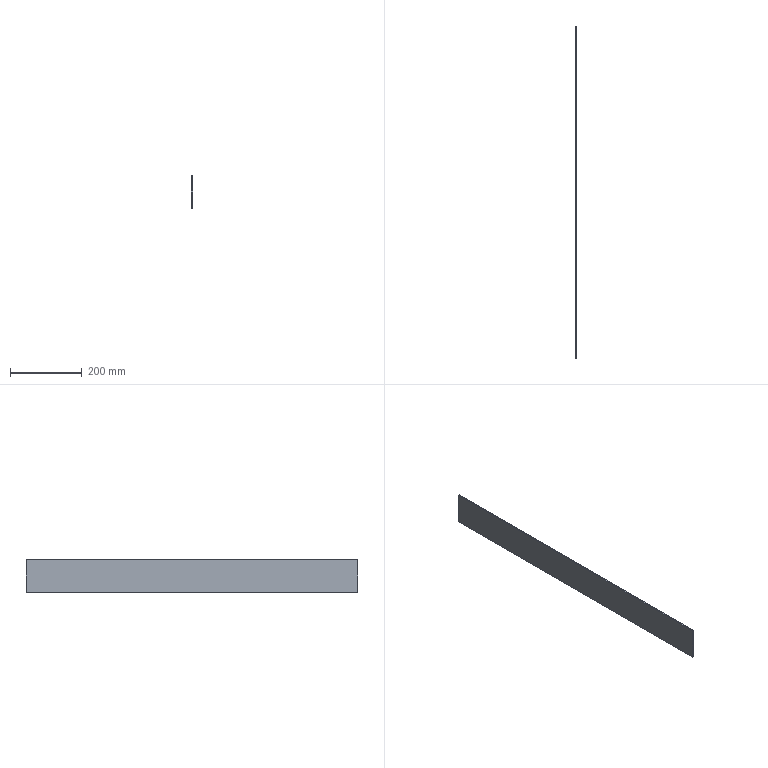Part | NX | features DATUM_CSYS 1, EXTRUDE 1, LINKED_CURVE 1 | 1 solid | 6 faces | box 3 x 926 x 90 mm | volume 250020 mm3 | plane 6
STEP:
#1=CARTESIAN_POINT('',(-455.,-463.,-88.163));
#2=VERTEX_POINT('',#1);
#3=CARTESIAN_POINT('',(-458.,-463.,-88.163));
#4=VERTEX_POINT('',#3);
#5=CARTESIAN_POINT('',(-455.,-463.,-88.163));
#6=DIRECTION('',(-1.,0.,0.));
#7=VECTOR('',#6,1000.);
#8=LINE('',#5,#7);
#9=EDGE_CURVE('',#2,#4,#8,.T.);
#10=ORIENTED_EDGE('',*,*,#9,.F.);
#11=CARTESIAN_POINT('',(-455.,-463.,1.837));
#12=VERTEX_POINT('',#11);
#13=CARTESIAN_POINT('',(-455.,-463.,-88.163));
#14=DIRECTION('',(0.,0.,1.));
#15=VECTOR('',#14,1000.);
#16=LINE('',#13,#15);
#17=EDGE_CURVE('',#2,#12,#16,.T.);
#18=ORIENTED_EDGE('',*,*,#17,.T.);
#19=CARTESIAN_POINT('',(-458.,-463.,1.837));
#20=VERTEX_POINT('',#19);
#21=CARTESIAN_POINT('',(-455.,-463.,1.837));
#22=DIRECTION('',(-1.,0.,0.));
#23=VECTOR('',#22,1000.);
#24=LINE('',#21,#23);
#25=EDGE_CURVE('',#12,#20,#24,.T.);
#26=ORIENTED_EDGE('',*,*,#25,.T.);
#27=CARTESIAN_POINT('',(-458.,-463.,-88.163));
#28=DIRECTION('',(0.,0.,1.));
#29=VECTOR('',#28,1000.);
#30=LINE('',#27,#29);
#31=EDGE_CURVE('',#4,#20,#30,.T.);
#32=ORIENTED_EDGE('',*,*,#31,.F.);
#33=EDGE_LOOP('',(#10,#18,#26,#32));
#34=FACE_BOUND('',#33,.T.);
#35=CARTESIAN_POINT('',(-455.,-463.,-88.163));
#36=DIRECTION('',(0.,-1.,0.));
#37=DIRECTION('',(0.,0.,1.));
#38=AXIS2_PLACEMENT_3D('',#35,#36,#37);
#39=PLANE('',#38);
#40=ADVANCED_FACE('',(#34),#39,.T.);
#41=ORIENTED_EDGE('',*,*,#25,.F.);
#42=CARTESIAN_POINT('',(-455.,463.,1.837));
#43=VERTEX_POINT('',#42);
#44=CARTESIAN_POINT('',(-455.,-463.,1.837));
#45=DIRECTION('',(0.,1.,0.));
#46=VECTOR('',#45,1000.);
#47=LINE('',#44,#46);
#48=EDGE_CURVE('',#12,#43,#47,.T.);
#49=ORIENTED_EDGE('',*,*,#48,.T.);
#50=CARTESIAN_POINT('',(-458.,463.,1.837));
#51=VERTEX_POINT('',#50);
#52=CARTESIAN_POINT('',(-455.,463.,1.837));
#53=DIRECTION('',(-1.,0.,0.));
#54=VECTOR('',#53,1000.);
#55=LINE('',#52,#54);
#56=EDGE_CURVE('',#43,#51,#55,.T.);
#57=ORIENTED_EDGE('',*,*,#56,.T.);
#58=CARTESIAN_POINT('',(-458.,-463.,1.837));
#59=DIRECTION('',(0.,1.,0.));
#60=VECTOR('',#59,1000.);
#61=LINE('',#58,#60);
#62=EDGE_CURVE('',#20,#51,#61,.T.);
#63=ORIENTED_EDGE('',*,*,#62,.F.);
#64=EDGE_LOOP('',(#41,#49,#57,#63));
#65=FACE_BOUND('',#64,.T.);
#66=CARTESIAN_POINT('',(-455.,-463.,1.837));
#67=DIRECTION('',(0.,0.,1.));
#68=DIRECTION('',(0.,1.,0.));
#69=AXIS2_PLACEMENT_3D('',#66,#67,#68);
#70=PLANE('',#69);
#71=ADVANCED_FACE('',(#65),#70,.T.);
#72=ORIENTED_EDGE('',*,*,#56,.F.);
#73=CARTESIAN_POINT('',(-455.,463.,-88.163));
#74=VERTEX_POINT('',#73);
#75=CARTESIAN_POINT('',(-455.,463.,-88.163));
#76=DIRECTION('',(0.,0.,1.));
#77=VECTOR('',#76,1000.);
#78=LINE('',#75,#77);
#79=EDGE_CURVE('',#74,#43,#78,.T.);
#80=ORIENTED_EDGE('',*,*,#79,.F.);
#81=CARTESIAN_POINT('',(-458.,463.,-88.163));
#82=VERTEX_POINT('',#81);
#83=CARTESIAN_POINT('',(-455.,463.,-88.163));
#84=DIRECTION('',(-1.,0.,0.));
#85=VECTOR('',#84,1000.);
#86=LINE('',#83,#85);
#87=EDGE_CURVE('',#74,#82,#86,.T.);
#88=ORIENTED_EDGE('',*,*,#87,.T.);
#89=CARTESIAN_POINT('',(-458.,463.,-88.163));
#90=DIRECTION('',(0.,0.,1.));
#91=VECTOR('',#90,1000.);
#92=LINE('',#89,#91);
#93=EDGE_CURVE('',#82,#51,#92,.T.);
#94=ORIENTED_EDGE('',*,*,#93,.T.);
#95=EDGE_LOOP('',(#72,#80,#88,#94));
#96=FACE_BOUND('',#95,.T.);
#97=CARTESIAN_POINT('',(-455.,463.,-88.163));
#98=DIRECTION('',(0.,-1.,0.));
#99=DIRECTION('',(0.,0.,1.));
#100=AXIS2_PLACEMENT_3D('',#97,#98,#99);
#101=PLANE('',#100);
#102=ADVANCED_FACE('',(#96),#101,.F.);
#103=CARTESIAN_POINT('',(-455.,-463.,-88.163));
#104=DIRECTION('',(0.,1.,0.));
#105=VECTOR('',#104,1000.);
#106=LINE('',#103,#105);
#107=EDGE_CURVE('',#2,#74,#106,.T.);
#108=ORIENTED_EDGE('',*,*,#107,.F.);
#109=ORIENTED_EDGE('',*,*,#9,.T.);
#110=CARTESIAN_POINT('',(-458.,-463.,-88.163));
#111=DIRECTION('',(0.,1.,0.));
#112=VECTOR('',#111,1000.);
#113=LINE('',#110,#112);
#114=EDGE_CURVE('',#4,#82,#113,.T.);
#115=ORIENTED_EDGE('',*,*,#114,.T.);
#116=ORIENTED_EDGE('',*,*,#87,.F.);
#117=EDGE_LOOP('',(#108,#109,#115,#116));
#118=FACE_BOUND('',#117,.T.);
#119=CARTESIAN_POINT('',(-455.,-463.,-88.163));
#120=DIRECTION('',(0.,0.,1.));
#121=DIRECTION('',(0.,1.,0.));
#122=AXIS2_PLACEMENT_3D('',#119,#120,#121);
#123=PLANE('',#122);
#124=ADVANCED_FACE('',(#118),#123,.F.);
#125=ORIENTED_EDGE('',*,*,#93,.F.);
#126=ORIENTED_EDGE('',*,*,#114,.F.);
#127=ORIENTED_EDGE('',*,*,#31,.T.);
#128=ORIENTED_EDGE('',*,*,#62,.T.);
#129=EDGE_LOOP('',(#125,#126,#127,#128));
#130=FACE_BOUND('',#129,.T.);
#131=CARTESIAN_POINT('',(-458.,-463.,-88.163));
#132=DIRECTION('',(-1.,0.,0.));
#133=DIRECTION('',(0.,0.,1.));
#134=AXIS2_PLACEMENT_3D('',#131,#132,#133);
#135=PLANE('',#134);
#136=ADVANCED_FACE('',(#130),#135,.T.);
#137=ORIENTED_EDGE('',*,*,#79,.T.);
#138=ORIENTED_EDGE('',*,*,#48,.F.);
#139=ORIENTED_EDGE('',*,*,#17,.F.);
#140=ORIENTED_EDGE('',*,*,#107,.T.);
#141=EDGE_LOOP('',(#137,#138,#139,#140));
#142=FACE_BOUND('',#141,.T.);
#143=CARTESIAN_POINT('',(-455.,-463.,-88.163));
#144=DIRECTION('',(-1.,0.,0.));
#145=DIRECTION('',(0.,0.,1.));
#146=AXIS2_PLACEMENT_3D('',#143,#144,#145);
#147=PLANE('',#146);
#148=ADVANCED_FACE('',(#142),#147,.F.);
#149=CLOSED_SHELL('',(#40,#71,#102,#124,#136,#148));
#150=MANIFOLD_SOLID_BREP('',#149);
#151=(LENGTH_UNIT()NAMED_UNIT(*)SI_UNIT(.MILLI.,.METRE.));
#152=UNCERTAINTY_MEASURE_WITH_UNIT(LENGTH_MEASURE(0.00001),#151,'','');
#153=(NAMED_UNIT(*)PLANE_ANGLE_UNIT()SI_UNIT($,.RADIAN.));
#154=(NAMED_UNIT(*)SI_UNIT($,.STERADIAN.)SOLID_ANGLE_UNIT());
#155=(GEOMETRIC_REPRESENTATION_CONTEXT(3)GLOBAL_UNCERTAINTY_ASSIGNED_CONTEXT((#152))GLOBAL_UNIT_ASSIGNED_CONTEXT((#151,#153,#154))REPRESENTATION_CONTEXT('',''));
#156=ADVANCED_BREP_SHAPE_REPRESENTATION('',(#150),#155);